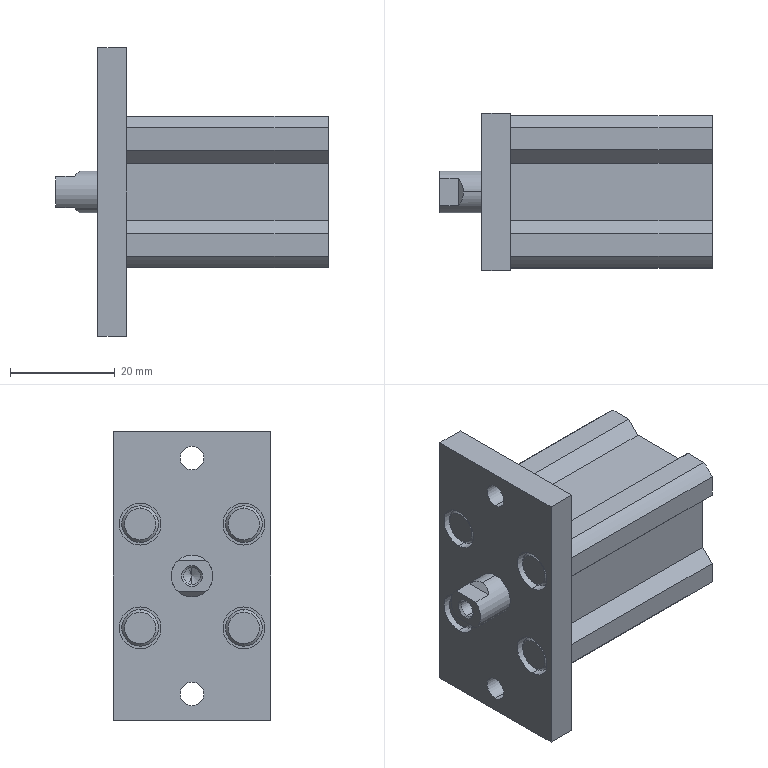Part | STEP file | CQ2F16-20D_0_0_0_ | 3 solids | 199 faces | box 52 x 30 x 55 mm | volume 31057 mm3 | cylinder 88 | plane 71 | cone 40 | commonest cylinder face diameters 3.242 x18 4 x16 8 x14 4.5 x12 7 x8 16 x8